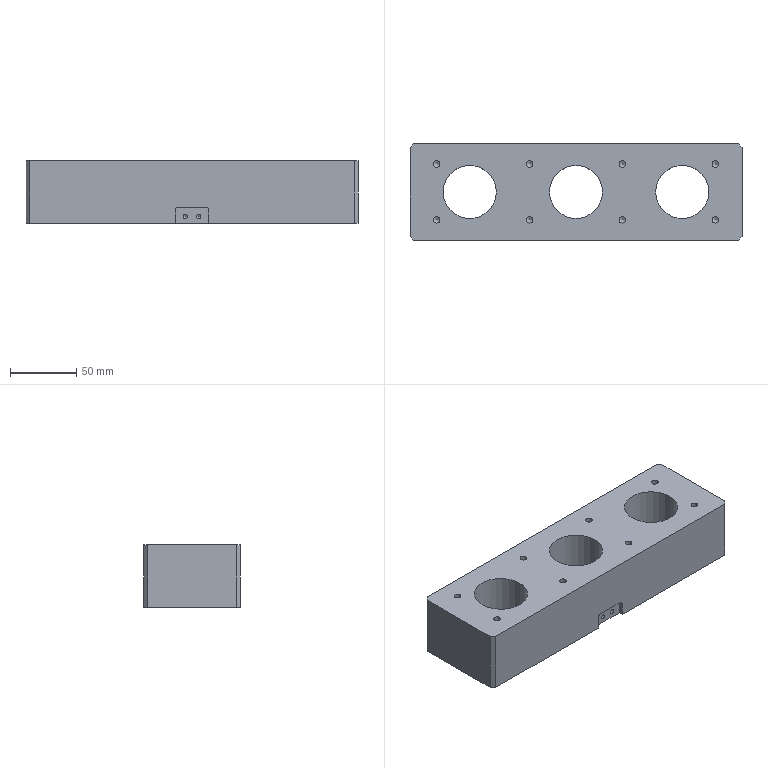Part | NX | 1 solid | 55 faces | box 250 x 73 x 47 mm | volume 670250 mm3 | cylinder 23 | cone 18 | plane 14 | commonest cylinder face diameters 5 x8 6.8 x8 40 x3 3.3 x2 4 x2
STEP:
#1=CARTESIAN_POINT('',(12.5,-36.5,0.));
#2=VERTEX_POINT('',#1);
#3=CARTESIAN_POINT('',(122.,-36.5,0.));
#4=VERTEX_POINT('',#3);
#5=CARTESIAN_POINT('',(125.,-36.5,0.));
#6=DIRECTION('',(1.,0.,0.));
#7=VECTOR('',#6,1000.);
#8=LINE('',#5,#7);
#9=EDGE_CURVE('',#2,#4,#8,.T.);
#10=ORIENTED_EDGE('',*,*,#9,.T.);
#11=CARTESIAN_POINT('',(122.,-36.5,47.));
#12=VERTEX_POINT('',#11);
#13=CARTESIAN_POINT('',(122.,-36.5,47.));
#14=DIRECTION('',(0.,0.,1.));
#15=VECTOR('',#14,1000.);
#16=LINE('',#13,#15);
#17=EDGE_CURVE('',#4,#12,#16,.T.);
#18=ORIENTED_EDGE('',*,*,#17,.T.);
#19=CARTESIAN_POINT('',(-122.,-36.5,47.));
#20=VERTEX_POINT('',#19);
#21=CARTESIAN_POINT('',(125.,-36.5,47.));
#22=DIRECTION('',(1.,0.,0.));
#23=VECTOR('',#22,1000.);
#24=LINE('',#21,#23);
#25=EDGE_CURVE('',#20,#12,#24,.T.);
#26=ORIENTED_EDGE('',*,*,#25,.F.);
#27=CARTESIAN_POINT('',(-122.,-36.5,0.));
#28=VERTEX_POINT('',#27);
#29=CARTESIAN_POINT('',(-122.,-36.5,47.));
#30=DIRECTION('',(0.,0.,-1.));
#31=VECTOR('',#30,1000.);
#32=LINE('',#29,#31);
#33=EDGE_CURVE('',#20,#28,#32,.T.);
#34=ORIENTED_EDGE('',*,*,#33,.T.);
#35=CARTESIAN_POINT('',(-12.5,-36.5,0.));
#36=VERTEX_POINT('',#35);
#37=CARTESIAN_POINT('',(125.,-36.5,0.));
#38=DIRECTION('',(1.,0.,0.));
#39=VECTOR('',#38,1000.);
#40=LINE('',#37,#39);
#41=EDGE_CURVE('',#28,#36,#40,.T.);
#42=ORIENTED_EDGE('',*,*,#41,.T.);
#43=CARTESIAN_POINT('',(-12.5,-36.5,10.));
#44=VERTEX_POINT('',#43);
#45=CARTESIAN_POINT('',(-12.5,-36.5,-12.));
#46=DIRECTION('',(0.,0.,1.));
#47=VECTOR('',#46,1000.);
#48=LINE('',#45,#47);
#49=EDGE_CURVE('',#36,#44,#48,.T.);
#50=ORIENTED_EDGE('',*,*,#49,.T.);
#51=CARTESIAN_POINT('',(-10.5,-36.5,12.));
#52=VERTEX_POINT('',#51);
#53=CARTESIAN_POINT('',(-10.5,-36.5,10.));
#54=DIRECTION('',(0.,1.,0.));
#55=DIRECTION('',(-1.,0.,0.));
#56=AXIS2_PLACEMENT_3D('',#53,#54,#55);
#57=CIRCLE('',#56,2.);
#58=EDGE_CURVE('',#44,#52,#57,.T.);
#59=ORIENTED_EDGE('',*,*,#58,.T.);
#60=CARTESIAN_POINT('',(10.5,-36.5,12.));
#61=VERTEX_POINT('',#60);
#62=CARTESIAN_POINT('',(12.5,-36.5,12.));
#63=DIRECTION('',(1.,0.,0.));
#64=VECTOR('',#63,1000.);
#65=LINE('',#62,#64);
#66=EDGE_CURVE('',#52,#61,#65,.T.);
#67=ORIENTED_EDGE('',*,*,#66,.T.);
#68=CARTESIAN_POINT('',(12.5,-36.5,10.));
#69=VERTEX_POINT('',#68);
#70=CARTESIAN_POINT('',(10.5,-36.5,10.));
#71=DIRECTION('',(0.,1.,0.));
#72=DIRECTION('',(-1.,0.,0.));
#73=AXIS2_PLACEMENT_3D('',#70,#71,#72);
#74=CIRCLE('',#73,2.);
#75=EDGE_CURVE('',#61,#69,#74,.T.);
#76=ORIENTED_EDGE('',*,*,#75,.T.);
#77=CARTESIAN_POINT('',(12.5,-36.5,-12.));
#78=DIRECTION('',(0.,0.,-1.));
#79=VECTOR('',#78,1000.);
#80=LINE('',#77,#79);
#81=EDGE_CURVE('',#69,#2,#80,.T.);
#82=ORIENTED_EDGE('',*,*,#81,.T.);
#83=EDGE_LOOP('',(#10,#18,#26,#34,#42,#50,#59,#67,#76,#82));
#84=FACE_BOUND('',#83,.T.);
#85=CARTESIAN_POINT('',(125.,-36.5,47.));
#86=DIRECTION('',(0.,1.,0.));
#87=DIRECTION('',(-1.,0.,0.));
#88=AXIS2_PLACEMENT_3D('',#85,#86,#87);
#89=PLANE('',#88);
#90=ADVANCED_FACE('',(#84),#89,.F.);
#91=CARTESIAN_POINT('',(102.1,-28.5,0.));
#92=VERTEX_POINT('',#91);
#93=CARTESIAN_POINT('',(105.5,-28.5,0.));
#94=DIRECTION('',(0.,0.,-1.));
#95=DIRECTION('',(-1.,0.,0.));
#96=AXIS2_PLACEMENT_3D('',#93,#94,#95);
#97=CIRCLE('',#96,3.4);
#98=EDGE_CURVE('',#92,#92,#97,.T.);
#99=ORIENTED_EDGE('',*,*,#98,.F.);
#100=EDGE_LOOP('',(#99));
#101=FACE_BOUND('',#100,.T.);
#102=CARTESIAN_POINT('',(57.1,-28.5,0.));
#103=VERTEX_POINT('',#102);
#104=CARTESIAN_POINT('',(60.5,-28.5,0.));
#105=DIRECTION('',(0.,0.,-1.));
#106=DIRECTION('',(-1.,0.,0.));
#107=AXIS2_PLACEMENT_3D('',#104,#105,#106);
#108=CIRCLE('',#107,3.4);
#109=EDGE_CURVE('',#103,#103,#108,.T.);
#110=ORIENTED_EDGE('',*,*,#109,.F.);
#111=EDGE_LOOP('',(#110));
#112=FACE_BOUND('',#111,.T.);
#113=CARTESIAN_POINT('',(-63.9,-28.5,0.));
#114=VERTEX_POINT('',#113);
#115=CARTESIAN_POINT('',(-60.5,-28.5,0.));
#116=DIRECTION('',(0.,0.,-1.));
#117=DIRECTION('',(-1.,0.,0.));
#118=AXIS2_PLACEMENT_3D('',#115,#116,#117);
#119=CIRCLE('',#118,3.4);
#120=EDGE_CURVE('',#114,#114,#119,.T.);
#121=ORIENTED_EDGE('',*,*,#120,.F.);
#122=EDGE_LOOP('',(#121));
#123=FACE_BOUND('',#122,.T.);
#124=CARTESIAN_POINT('',(-108.9,-28.5,0.));
#125=VERTEX_POINT('',#124);
#126=CARTESIAN_POINT('',(-105.5,-28.5,0.));
#127=DIRECTION('',(0.,0.,-1.));
#128=DIRECTION('',(-1.,0.,0.));
#129=AXIS2_PLACEMENT_3D('',#126,#127,#128);
#130=CIRCLE('',#129,3.4);
#131=EDGE_CURVE('',#125,#125,#130,.T.);
#132=ORIENTED_EDGE('',*,*,#131,.F.);
#133=EDGE_LOOP('',(#132));
#134=FACE_BOUND('',#133,.T.);
#135=CARTESIAN_POINT('',(-108.9,28.5,0.));
#136=VERTEX_POINT('',#135);
#137=CARTESIAN_POINT('',(-105.5,28.5,0.));
#138=DIRECTION('',(0.,0.,-1.));
#139=DIRECTION('',(-1.,0.,0.));
#140=AXIS2_PLACEMENT_3D('',#137,#138,#139);
#141=CIRCLE('',#140,3.4);
#142=EDGE_CURVE('',#136,#136,#141,.T.);
#143=ORIENTED_EDGE('',*,*,#142,.F.);
#144=EDGE_LOOP('',(#143));
#145=FACE_BOUND('',#144,.T.);
#146=CARTESIAN_POINT('',(-63.9,28.5,0.));
#147=VERTEX_POINT('',#146);
#148=CARTESIAN_POINT('',(-60.5,28.5,0.));
#149=DIRECTION('',(0.,0.,-1.));
#150=DIRECTION('',(-1.,0.,0.));
#151=AXIS2_PLACEMENT_3D('',#148,#149,#150);
#152=CIRCLE('',#151,3.4);
#153=EDGE_CURVE('',#147,#147,#152,.T.);
#154=ORIENTED_EDGE('',*,*,#153,.F.);
#155=EDGE_LOOP('',(#154));
#156=FACE_BOUND('',#155,.T.);
#157=CARTESIAN_POINT('',(57.1,28.5,0.));
#158=VERTEX_POINT('',#157);
#159=CARTESIAN_POINT('',(60.5,28.5,0.));
#160=DIRECTION('',(0.,0.,-1.));
#161=DIRECTION('',(-1.,0.,0.));
#162=AXIS2_PLACEMENT_3D('',#159,#160,#161);
#163=CIRCLE('',#162,3.4);
#164=EDGE_CURVE('',#158,#158,#163,.T.);
#165=ORIENTED_EDGE('',*,*,#164,.F.);
#166=EDGE_LOOP('',(#165));
#167=FACE_BOUND('',#166,.T.);
#168=CARTESIAN_POINT('',(102.1,28.5,0.));
#169=VERTEX_POINT('',#168);
#170=CARTESIAN_POINT('',(105.5,28.5,0.));
#171=DIRECTION('',(0.,0.,-1.));
#172=DIRECTION('',(-1.,0.,0.));
#173=AXIS2_PLACEMENT_3D('',#170,#171,#172);
#174=CIRCLE('',#173,3.4);
#175=EDGE_CURVE('',#169,#169,#174,.T.);
#176=ORIENTED_EDGE('',*,*,#175,.F.);
#177=EDGE_LOOP('',(#176));
#178=FACE_BOUND('',#177,.T.);
#179=CARTESIAN_POINT('',(-20.,0.,0.));
#180=VERTEX_POINT('',#179);
#181=CARTESIAN_POINT('',(0.,0.,0.));
#182=DIRECTION('',(0.,0.,-1.));
#183=DIRECTION('',(-1.,0.,0.));
#184=AXIS2_PLACEMENT_3D('',#181,#182,#183);
#185=CIRCLE('',#184,20.);
#186=EDGE_CURVE('',#180,#180,#185,.T.);
#187=ORIENTED_EDGE('',*,*,#186,.F.);
#188=EDGE_LOOP('',(#187));
#189=FACE_BOUND('',#188,.T.);
#190=CARTESIAN_POINT('',(-100.,0.,0.));
#191=VERTEX_POINT('',#190);
#192=CARTESIAN_POINT('',(-80.,0.,0.));
#193=DIRECTION('',(0.,0.,-1.));
#194=DIRECTION('',(-1.,0.,0.));
#195=AXIS2_PLACEMENT_3D('',#192,#193,#194);
#196=CIRCLE('',#195,20.);
#197=EDGE_CURVE('',#191,#191,#196,.T.);
#198=ORIENTED_EDGE('',*,*,#197,.F.);
#199=EDGE_LOOP('',(#198));
#200=FACE_BOUND('',#199,.T.);
#201=CARTESIAN_POINT('',(60.,0.,0.));
#202=VERTEX_POINT('',#201);
#203=CARTESIAN_POINT('',(80.,0.,0.));
#204=DIRECTION('',(0.,0.,-1.));
#205=DIRECTION('',(-1.,0.,0.));
#206=AXIS2_PLACEMENT_3D('',#203,#204,#205);
#207=CIRCLE('',#206,20.);
#208=EDGE_CURVE('',#202,#202,#207,.T.);
#209=ORIENTED_EDGE('',*,*,#208,.F.);
#210=EDGE_LOOP('',(#209));
#211=FACE_BOUND('',#210,.T.);
#212=CARTESIAN_POINT('',(122.,36.5,0.));
#213=VERTEX_POINT('',#212);
#214=CARTESIAN_POINT('',(-122.,36.5,0.));
#215=VERTEX_POINT('',#214);
#216=CARTESIAN_POINT('',(125.,36.5,0.));
#217=DIRECTION('',(-1.,0.,0.));
#218=VECTOR('',#217,1000.);
#219=LINE('',#216,#218);
#220=EDGE_CURVE('',#213,#215,#219,.T.);
#221=ORIENTED_EDGE('',*,*,#220,.F.);
#222=CARTESIAN_POINT('',(125.,33.5,0.));
#223=VERTEX_POINT('',#222);
#224=CARTESIAN_POINT('',(79.25,79.25,0.));
#225=DIRECTION('',(-0.7071,0.7071,0.));
#226=VECTOR('',#225,1000.);
#227=LINE('',#224,#226);
#228=EDGE_CURVE('',#213,#223,#227,.F.);
#229=ORIENTED_EDGE('',*,*,#228,.T.);
#230=CARTESIAN_POINT('',(125.,-33.5,0.));
#231=VERTEX_POINT('',#230);
#232=CARTESIAN_POINT('',(125.,36.5,0.));
#233=DIRECTION('',(0.,1.,0.));
#234=VECTOR('',#233,1000.);
#235=LINE('',#232,#234);
#236=EDGE_CURVE('',#231,#223,#235,.T.);
#237=ORIENTED_EDGE('',*,*,#236,.F.);
#238=CARTESIAN_POINT('',(79.25,-79.25,0.));
#239=DIRECTION('',(0.7071,0.7071,0.));
#240=VECTOR('',#239,1000.);
#241=LINE('',#238,#240);
#242=EDGE_CURVE('',#231,#4,#241,.F.);
#243=ORIENTED_EDGE('',*,*,#242,.T.);
#244=ORIENTED_EDGE('',*,*,#9,.F.);
#245=CARTESIAN_POINT('',(12.5,-33.5,0.));
#246=VERTEX_POINT('',#245);
#247=CARTESIAN_POINT('',(12.5,0.,0.));
#248=DIRECTION('',(0.,1.,0.));
#249=VECTOR('',#248,1000.);
#250=LINE('',#247,#249);
#251=EDGE_CURVE('',#2,#246,#250,.T.);
#252=ORIENTED_EDGE('',*,*,#251,.T.);
#253=CARTESIAN_POINT('',(-12.5,-33.5,0.));
#254=VERTEX_POINT('',#253);
#255=CARTESIAN_POINT('',(0.,-33.5,0.));
#256=DIRECTION('',(-1.,0.,0.));
#257=VECTOR('',#256,1000.);
#258=LINE('',#255,#257);
#259=EDGE_CURVE('',#246,#254,#258,.T.);
#260=ORIENTED_EDGE('',*,*,#259,.T.);
#261=CARTESIAN_POINT('',(-12.5,0.,0.));
#262=DIRECTION('',(0.,-1.,0.));
#263=VECTOR('',#262,1000.);
#264=LINE('',#261,#263);
#265=EDGE_CURVE('',#254,#36,#264,.T.);
#266=ORIENTED_EDGE('',*,*,#265,.T.);
#267=ORIENTED_EDGE('',*,*,#41,.F.);
#268=CARTESIAN_POINT('',(-125.,-33.5,0.));
#269=VERTEX_POINT('',#268);
#270=CARTESIAN_POINT('',(-79.25,-79.25,0.));
#271=DIRECTION('',(0.7071,-0.7071,0.));
#272=VECTOR('',#271,1000.);
#273=LINE('',#270,#272);
#274=EDGE_CURVE('',#28,#269,#273,.F.);
#275=ORIENTED_EDGE('',*,*,#274,.T.);
#276=CARTESIAN_POINT('',(-125.,33.5,0.));
#277=VERTEX_POINT('',#276);
#278=CARTESIAN_POINT('',(-125.,36.5,0.));
#279=DIRECTION('',(0.,-1.,0.));
#280=VECTOR('',#279,1000.);
#281=LINE('',#278,#280);
#282=EDGE_CURVE('',#277,#269,#281,.T.);
#283=ORIENTED_EDGE('',*,*,#282,.F.);
#284=CARTESIAN_POINT('',(-79.25,79.25,0.));
#285=DIRECTION('',(-0.7071,-0.7071,0.));
#286=VECTOR('',#285,1000.);
#287=LINE('',#284,#286);
#288=EDGE_CURVE('',#277,#215,#287,.F.);
#289=ORIENTED_EDGE('',*,*,#288,.T.);
#290=EDGE_LOOP('',(#221,#229,#237,#243,#244,#252,#260,#266,#267,#275,#283,#289));
#291=FACE_BOUND('',#290,.T.);
#292=CARTESIAN_POINT('',(0.,0.,0.));
#293=DIRECTION('',(0.,0.,-1.));
#294=DIRECTION('',(-1.,0.,0.));
#295=AXIS2_PLACEMENT_3D('',#292,#293,#294);
#296=PLANE('',#295);
#297=ADVANCED_FACE('',(#101,#112,#123,#134,#145,#156,#167,#178,#189,#200,#211,#291),#296,.T.);
#298=CARTESIAN_POINT('',(-125.,33.5,47.));
#299=VERTEX_POINT('',#298);
#300=CARTESIAN_POINT('',(-125.,-33.5,47.));
#301=VERTEX_POINT('',#300);
#302=CARTESIAN_POINT('',(-125.,36.5,47.));
#303=DIRECTION('',(0.,-1.,0.));
#304=VECTOR('',#303,1000.);
#305=LINE('',#302,#304);
#306=EDGE_CURVE('',#299,#301,#305,.T.);
#307=ORIENTED_EDGE('',*,*,#306,.F.);
#308=CARTESIAN_POINT('',(-125.,33.5,47.));
#309=DIRECTION('',(0.,0.,-1.));
#310=VECTOR('',#309,1000.);
#311=LINE('',#308,#310);
#312=EDGE_CURVE('',#299,#277,#311,.T.);
#313=ORIENTED_EDGE('',*,*,#312,.T.);
#314=ORIENTED_EDGE('',*,*,#282,.T.);
#315=CARTESIAN_POINT('',(-125.,-33.5,47.));
#316=DIRECTION('',(0.,0.,1.));
#317=VECTOR('',#316,1000.);
#318=LINE('',#315,#317);
#319=EDGE_CURVE('',#269,#301,#318,.T.);
#320=ORIENTED_EDGE('',*,*,#319,.T.);
#321=EDGE_LOOP('',(#307,#313,#314,#320));
#322=FACE_BOUND('',#321,.T.);
#323=CARTESIAN_POINT('',(-125.,36.5,47.));
#324=DIRECTION('',(1.,0.,0.));
#325=DIRECTION('',(0.,1.,0.));
#326=AXIS2_PLACEMENT_3D('',#323,#324,#325);
#327=PLANE('',#326);
#328=ADVANCED_FACE('',(#322),#327,.F.);
#329=ORIENTED_EDGE('',*,*,#236,.T.);
#330=CARTESIAN_POINT('',(125.,33.5,47.));
#331=VERTEX_POINT('',#330);
#332=CARTESIAN_POINT('',(125.,33.5,47.));
#333=DIRECTION('',(0.,0.,1.));
#334=VECTOR('',#333,1000.);
#335=LINE('',#332,#334);
#336=EDGE_CURVE('',#223,#331,#335,.T.);
#337=ORIENTED_EDGE('',*,*,#336,.T.);
#338=CARTESIAN_POINT('',(125.,-33.5,47.));
#339=VERTEX_POINT('',#338);
#340=CARTESIAN_POINT('',(125.,36.5,47.));
#341=DIRECTION('',(0.,1.,0.));
#342=VECTOR('',#341,1000.);
#343=LINE('',#340,#342);
#344=EDGE_CURVE('',#339,#331,#343,.T.);
#345=ORIENTED_EDGE('',*,*,#344,.F.);
#346=CARTESIAN_POINT('',(125.,-33.5,47.));
#347=DIRECTION('',(0.,0.,-1.));
#348=VECTOR('',#347,1000.);
#349=LINE('',#346,#348);
#350=EDGE_CURVE('',#339,#231,#349,.T.);
#351=ORIENTED_EDGE('',*,*,#350,.T.);
#352=EDGE_LOOP('',(#329,#337,#345,#351));
#353=FACE_BOUND('',#352,.T.);
#354=CARTESIAN_POINT('',(125.,36.5,47.));
#355=DIRECTION('',(-1.,0.,0.));
#356=DIRECTION('',(0.,0.,1.));
#357=AXIS2_PLACEMENT_3D('',#354,#355,#356);
#358=PLANE('',#357);
#359=ADVANCED_FACE('',(#353),#358,.F.);
#360=CARTESIAN_POINT('',(122.,36.5,47.));
#361=VERTEX_POINT('',#360);
#362=CARTESIAN_POINT('',(-122.,36.5,47.));
#363=VERTEX_POINT('',#362);
#364=CARTESIAN_POINT('',(125.,36.5,47.));
#365=DIRECTION('',(-1.,0.,0.));
#366=VECTOR('',#365,1000.);
#367=LINE('',#364,#366);
#368=EDGE_CURVE('',#361,#363,#367,.T.);
#369=ORIENTED_EDGE('',*,*,#368,.F.);
#370=CARTESIAN_POINT('',(122.,36.5,47.));
#371=DIRECTION('',(0.,0.,-1.));
#372=VECTOR('',#371,1000.);
#373=LINE('',#370,#372);
#374=EDGE_CURVE('',#361,#213,#373,.T.);
#375=ORIENTED_EDGE('',*,*,#374,.T.);
#376=ORIENTED_EDGE('',*,*,#220,.T.);
#377=CARTESIAN_POINT('',(-122.,36.5,47.));
#378=DIRECTION('',(0.,0.,1.));
#379=VECTOR('',#378,1000.);
#380=LINE('',#377,#379);
#381=EDGE_CURVE('',#215,#363,#380,.T.);
#382=ORIENTED_EDGE('',*,*,#381,.T.);
#383=EDGE_LOOP('',(#369,#375,#376,#382));
#384=FACE_BOUND('',#383,.T.);
#385=CARTESIAN_POINT('',(125.,36.5,47.));
#386=DIRECTION('',(0.,-1.,0.));
#387=DIRECTION('',(1.,0.,0.));
#388=AXIS2_PLACEMENT_3D('',#385,#386,#387);
#389=PLANE('',#388);
#390=ADVANCED_FACE('',(#384),#389,.F.);
#391=CARTESIAN_POINT('',(60.,0.,47.));
#392=VERTEX_POINT('',#391);
#393=CARTESIAN_POINT('',(80.,0.,47.));
#394=DIRECTION('',(0.,0.,-1.));
#395=DIRECTION('',(-1.,0.,0.));
#396=AXIS2_PLACEMENT_3D('',#393,#394,#395);
#397=CIRCLE('',#396,20.);
#398=EDGE_CURVE('',#392,#392,#397,.T.);
#399=ORIENTED_EDGE('',*,*,#398,.T.);
#400=EDGE_LOOP('',(#399));
#401=FACE_BOUND('',#400,.T.);
#402=CARTESIAN_POINT('',(-100.,0.,47.));
#403=VERTEX_POINT('',#402);
#404=CARTESIAN_POINT('',(-80.,0.,47.));
#405=DIRECTION('',(0.,0.,-1.));
#406=DIRECTION('',(-1.,0.,0.));
#407=AXIS2_PLACEMENT_3D('',#404,#405,#406);
#408=CIRCLE('',#407,20.);
#409=EDGE_CURVE('',#403,#403,#408,.T.);
#410=ORIENTED_EDGE('',*,*,#409,.T.);
#411=EDGE_LOOP('',(#410));
#412=FACE_BOUND('',#411,.T.);
#413=CARTESIAN_POINT('',(-20.,0.,47.));
#414=VERTEX_POINT('',#413);
#415=CARTESIAN_POINT('',(0.,0.,47.));
#416=DIRECTION('',(0.,0.,-1.));
#417=DIRECTION('',(-1.,0.,0.));
#418=AXIS2_PLACEMENT_3D('',#415,#416,#417);
#419=CIRCLE('',#418,20.);
#420=EDGE_CURVE('',#414,#414,#419,.T.);
#421=ORIENTED_EDGE('',*,*,#420,.T.);
#422=EDGE_LOOP('',(#421));
#423=FACE_BOUND('',#422,.T.);
#424=CARTESIAN_POINT('',(-102.5,21.,47.));
#425=VERTEX_POINT('',#424);
#426=CARTESIAN_POINT('',(-105.,21.,47.));
#427=DIRECTION('',(0.,0.,1.));
#428=DIRECTION('',(1.,0.,0.));
#429=AXIS2_PLACEMENT_3D('',#426,#427,#428);
#430=CIRCLE('',#429,2.5);
#431=EDGE_CURVE('',#425,#425,#430,.T.);
#432=ORIENTED_EDGE('',*,*,#431,.F.);
#433=EDGE_LOOP('',(#432));
#434=FACE_BOUND('',#433,.T.);
#435=CARTESIAN_POINT('',(-32.5,21.,47.));
#436=VERTEX_POINT('',#435);
#437=CARTESIAN_POINT('',(-35.,21.,47.));
#438=DIRECTION('',(0.,0.,1.));
#439=DIRECTION('',(1.,0.,0.));
#440=AXIS2_PLACEMENT_3D('',#437,#438,#439);
#441=CIRCLE('',#440,2.5);
#442=EDGE_CURVE('',#436,#436,#441,.T.);
#443=ORIENTED_EDGE('',*,*,#442,.F.);
#444=EDGE_LOOP('',(#443));
#445=FACE_BOUND('',#444,.T.);
#446=CARTESIAN_POINT('',(-32.5,-21.,47.));
#447=VERTEX_POINT('',#446);
#448=CARTESIAN_POINT('',(-35.,-21.,47.));
#449=DIRECTION('',(0.,0.,1.));
#450=DIRECTION('',(1.,0.,0.));
#451=AXIS2_PLACEMENT_3D('',#448,#449,#450);
#452=CIRCLE('',#451,2.5);
#453=EDGE_CURVE('',#447,#447,#452,.T.);
#454=ORIENTED_EDGE('',*,*,#453,.F.);
#455=EDGE_LOOP('',(#454));
#456=FACE_BOUND('',#455,.T.);
#457=CARTESIAN_POINT('',(-102.5,-21.,47.));
#458=VERTEX_POINT('',#457);
#459=CARTESIAN_POINT('',(-105.,-21.,47.));
#460=DIRECTION('',(0.,0.,1.));
#461=DIRECTION('',(1.,0.,0.));
#462=AXIS2_PLACEMENT_3D('',#459,#460,#461);
#463=CIRCLE('',#462,2.5);
#464=EDGE_CURVE('',#458,#458,#463,.T.);
#465=ORIENTED_EDGE('',*,*,#464,.F.);
#466=EDGE_LOOP('',(#465));
#467=FACE_BOUND('',#466,.T.);
#468=CARTESIAN_POINT('',(107.5,-21.,47.));
#469=VERTEX_POINT('',#468);
#470=CARTESIAN_POINT('',(105.,-21.,47.));
#471=DIRECTION('',(0.,0.,1.));
#472=DIRECTION('',(1.,0.,0.));
#473=AXIS2_PLACEMENT_3D('',#470,#471,#472);
#474=CIRCLE('',#473,2.5);
#475=EDGE_CURVE('',#469,#469,#474,.T.);
#476=ORIENTED_EDGE('',*,*,#475,.F.);
#477=EDGE_LOOP('',(#476));
#478=FACE_BOUND('',#477,.T.);
#479=CARTESIAN_POINT('',(37.5,-21.,47.));
#480=VERTEX_POINT('',#479);
#481=CARTESIAN_POINT('',(35.,-21.,47.));
#482=DIRECTION('',(0.,0.,1.));
#483=DIRECTION('',(1.,0.,0.));
#484=AXIS2_PLACEMENT_3D('',#481,#482,#483);
#485=CIRCLE('',#484,2.5);
#486=EDGE_CURVE('',#480,#480,#485,.T.);
#487=ORIENTED_EDGE('',*,*,#486,.F.);
#488=EDGE_LOOP('',(#487));
#489=FACE_BOUND('',#488,.T.);
#490=CARTESIAN_POINT('',(37.5,21.,47.));
#491=VERTEX_POINT('',#490);
#492=CARTESIAN_POINT('',(35.,21.,47.));
#493=DIRECTION('',(0.,0.,1.));
#494=DIRECTION('',(1.,0.,0.));
#495=AXIS2_PLACEMENT_3D('',#492,#493,#494);
#496=CIRCLE('',#495,2.5);
#497=EDGE_CURVE('',#491,#491,#496,.T.);
#498=ORIENTED_EDGE('',*,*,#497,.F.);
#499=EDGE_LOOP('',(#498));
#500=FACE_BOUND('',#499,.T.);
#501=CARTESIAN_POINT('',(107.5,21.,47.));
#502=VERTEX_POINT('',#501);
#503=CARTESIAN_POINT('',(105.,21.,47.));
#504=DIRECTION('',(0.,0.,1.));
#505=DIRECTION('',(1.,0.,0.));
#506=AXIS2_PLACEMENT_3D('',#503,#504,#505);
#507=CIRCLE('',#506,2.5);
#508=EDGE_CURVE('',#502,#502,#507,.T.);
#509=ORIENTED_EDGE('',*,*,#508,.F.);
#510=EDGE_LOOP('',(#509));
#511=FACE_BOUND('',#510,.T.);
#512=ORIENTED_EDGE('',*,*,#344,.T.);
#513=CARTESIAN_POINT('',(122.,36.5,47.));
#514=DIRECTION('',(0.7071,-0.7071,0.));
#515=VECTOR('',#514,1000.);
#516=LINE('',#513,#515);
#517=EDGE_CURVE('',#331,#361,#516,.F.);
#518=ORIENTED_EDGE('',*,*,#517,.T.);
#519=ORIENTED_EDGE('',*,*,#368,.T.);
#520=CARTESIAN_POINT('',(-125.,33.5,47.));
#521=DIRECTION('',(0.7071,0.7071,0.));
#522=VECTOR('',#521,1000.);
#523=LINE('',#520,#522);
#524=EDGE_CURVE('',#363,#299,#523,.F.);
#525=ORIENTED_EDGE('',*,*,#524,.T.);
#526=ORIENTED_EDGE('',*,*,#306,.T.);
#527=CARTESIAN_POINT('',(-122.,-36.5,47.));
#528=DIRECTION('',(-0.7071,0.7071,0.));
#529=VECTOR('',#528,1000.);
#530=LINE('',#527,#529);
#531=EDGE_CURVE('',#301,#20,#530,.F.);
#532=ORIENTED_EDGE('',*,*,#531,.T.);
#533=ORIENTED_EDGE('',*,*,#25,.T.);
#534=CARTESIAN_POINT('',(125.,-33.5,47.));
#535=DIRECTION('',(-0.7071,-0.7071,0.));
#536=VECTOR('',#535,1000.);
#537=LINE('',#534,#536);
#538=EDGE_CURVE('',#12,#339,#537,.F.);
#539=ORIENTED_EDGE('',*,*,#538,.T.);
#540=EDGE_LOOP('',(#512,#518,#519,#525,#526,#532,#533,#539));
#541=FACE_BOUND('',#540,.T.);
#542=CARTESIAN_POINT('',(0.,0.,47.));
#543=DIRECTION('',(0.,0.,-1.));
#544=DIRECTION('',(-1.,0.,0.));
#545=AXIS2_PLACEMENT_3D('',#542,#543,#544);
#546=PLANE('',#545);
#547=ADVANCED_FACE('',(#401,#412,#423,#434,#445,#456,#467,#478,#489,#500,#511,#541),#546,.F.);
#548=CARTESIAN_POINT('',(105.5,-28.5,21.793));
#549=VERTEX_POINT('',#548);
#550=VERTEX_LOOP('',#549);
#551=FACE_BOUND('',#550,.T.);
#552=CARTESIAN_POINT('',(102.1,-28.5,19.75));
#553=VERTEX_POINT('',#552);
#554=CARTESIAN_POINT('',(105.5,-28.5,19.75));
#555=DIRECTION('',(0.,0.,-1.));
#556=DIRECTION('',(-1.,0.,0.));
#557=AXIS2_PLACEMENT_3D('',#554,#555,#556);
#558=CIRCLE('',#557,3.4);
#559=EDGE_CURVE('',#553,#553,#558,.T.);
#560=ORIENTED_EDGE('',*,*,#559,.T.);
#561=EDGE_LOOP('',(#560));
#562=FACE_BOUND('',#561,.T.);
#563=CARTESIAN_POINT('',(105.5,-28.5,19.75));
#564=DIRECTION('',(0.,0.,-1.));
#565=DIRECTION('',(-1.,0.,0.));
#566=AXIS2_PLACEMENT_3D('',#563,#564,#565);
#567=CONICAL_SURFACE('',#566,3.4,1.03);
#568=ADVANCED_FACE('',(#551,#562),#567,.F.);
#569=ORIENTED_EDGE('',*,*,#559,.F.);
#570=EDGE_LOOP('',(#569));
#571=FACE_BOUND('',#570,.T.);
#572=ORIENTED_EDGE('',*,*,#98,.T.);
#573=EDGE_LOOP('',(#572));
#574=FACE_BOUND('',#573,.T.);
#575=CARTESIAN_POINT('',(105.5,-28.5,0.));
#576=DIRECTION('',(0.,0.,-1.));
#577=DIRECTION('',(-1.,0.,0.));
#578=AXIS2_PLACEMENT_3D('',#575,#576,#577);
#579=CYLINDRICAL_SURFACE('',#578,3.4);
#580=ADVANCED_FACE('',(#571,#574),#579,.F.);
#581=CARTESIAN_POINT('',(60.5,-28.5,21.793));
#582=VERTEX_POINT('',#581);
#583=VERTEX_LOOP('',#582);
#584=FACE_BOUND('',#583,.T.);
#585=CARTESIAN_POINT('',(57.1,-28.5,19.75));
#586=VERTEX_POINT('',#585);
#587=CARTESIAN_POINT('',(60.5,-28.5,19.75));
#588=DIRECTION('',(0.,0.,-1.));
#589=DIRECTION('',(-1.,0.,0.));
#590=AXIS2_PLACEMENT_3D('',#587,#588,#589);
#591=CIRCLE('',#590,3.4);
#592=EDGE_CURVE('',#586,#586,#591,.T.);
#593=ORIENTED_EDGE('',*,*,#592,.T.);
#594=EDGE_LOOP('',(#593));
#595=FACE_BOUND('',#594,.T.);
#596=CARTESIAN_POINT('',(60.5,-28.5,19.75));
#597=DIRECTION('',(0.,0.,-1.));
#598=DIRECTION('',(-1.,0.,0.));
#599=AXIS2_PLACEMENT_3D('',#596,#597,#598);
#600=CONICAL_SURFACE('',#599,3.4,1.03);
#601=ADVANCED_FACE('',(#584,#595),#600,.F.);
#602=ORIENTED_EDGE('',*,*,#592,.F.);
#603=EDGE_LOOP('',(#602));
#604=FACE_BOUND('',#603,.T.);
#605=ORIENTED_EDGE('',*,*,#109,.T.);
#606=EDGE_LOOP('',(#605));
#607=FACE_BOUND('',#606,.T.);
#608=CARTESIAN_POINT('',(60.5,-28.5,0.));
#609=DIRECTION('',(0.,0.,-1.));
#610=DIRECTION('',(-1.,0.,0.));
#611=AXIS2_PLACEMENT_3D('',#608,#609,#610);
#612=CYLINDRICAL_SURFACE('',#611,3.4);
#613=ADVANCED_FACE('',(#604,#607),#612,.F.);
#614=CARTESIAN_POINT('',(-60.5,-28.5,21.793));
#615=VERTEX_POINT('',#614);
#616=VERTEX_LOOP('',#615);
#617=FACE_BOUND('',#616,.T.);
#618=CARTESIAN_POINT('',(-63.9,-28.5,19.75));
#619=VERTEX_POINT('',#618);
#620=CARTESIAN_POINT('',(-60.5,-28.5,19.75));
#621=DIRECTION('',(0.,0.,-1.));
#622=DIRECTION('',(-1.,0.,0.));
#623=AXIS2_PLACEMENT_3D('',#620,#621,#622);
#624=CIRCLE('',#623,3.4);
#625=EDGE_CURVE('',#619,#619,#624,.T.);
#626=ORIENTED_EDGE('',*,*,#625,.T.);
#627=EDGE_LOOP('',(#626));
#628=FACE_BOUND('',#627,.T.);
#629=CARTESIAN_POINT('',(-60.5,-28.5,19.75));
#630=DIRECTION('',(0.,0.,-1.));
#631=DIRECTION('',(-1.,0.,0.));
#632=AXIS2_PLACEMENT_3D('',#629,#630,#631);
#633=CONICAL_SURFACE('',#632,3.4,1.03);
#634=ADVANCED_FACE('',(#617,#628),#633,.F.);
#635=ORIENTED_EDGE('',*,*,#625,.F.);
#636=EDGE_LOOP('',(#635));
#637=FACE_BOUND('',#636,.T.);
#638=ORIENTED_EDGE('',*,*,#120,.T.);
#639=EDGE_LOOP('',(#638));
#640=FACE_BOUND('',#639,.T.);
#641=CARTESIAN_POINT('',(-60.5,-28.5,0.));
#642=DIRECTION('',(0.,0.,-1.));
#643=DIRECTION('',(-1.,0.,0.));
#644=AXIS2_PLACEMENT_3D('',#641,#642,#643);
#645=CYLINDRICAL_SURFACE('',#644,3.4);
#646=ADVANCED_FACE('',(#637,#640),#645,.F.);
#647=CARTESIAN_POINT('',(-105.5,-28.5,21.793));
#648=VERTEX_POINT('',#647);
#649=VERTEX_LOOP('',#648);
#650=FACE_BOUND('',#649,.T.);
#651=CARTESIAN_POINT('',(-108.9,-28.5,19.75));
#652=VERTEX_POINT('',#651);
#653=CARTESIAN_POINT('',(-105.5,-28.5,19.75));
#654=DIRECTION('',(0.,0.,-1.));
#655=DIRECTION('',(-1.,0.,0.));
#656=AXIS2_PLACEMENT_3D('',#653,#654,#655);
#657=CIRCLE('',#656,3.4);
#658=EDGE_CURVE('',#652,#652,#657,.T.);
#659=ORIENTED_EDGE('',*,*,#658,.T.);
#660=EDGE_LOOP('',(#659));
#661=FACE_BOUND('',#660,.T.);
#662=CARTESIAN_POINT('',(-105.5,-28.5,19.75));
#663=DIRECTION('',(0.,0.,-1.));
#664=DIRECTION('',(-1.,0.,0.));
#665=AXIS2_PLACEMENT_3D('',#662,#663,#664);
#666=CONICAL_SURFACE('',#665,3.4,1.03);
#667=ADVANCED_FACE('',(#650,#661),#666,.F.);
#668=ORIENTED_EDGE('',*,*,#658,.F.);
#669=EDGE_LOOP('',(#668));
#670=FACE_BOUND('',#669,.T.);
#671=ORIENTED_EDGE('',*,*,#131,.T.);
#672=EDGE_LOOP('',(#671));
#673=FACE_BOUND('',#672,.T.);
#674=CARTESIAN_POINT('',(-105.5,-28.5,0.));
#675=DIRECTION('',(0.,0.,-1.));
#676=DIRECTION('',(-1.,0.,0.));
#677=AXIS2_PLACEMENT_3D('',#674,#675,#676);
#678=CYLINDRICAL_SURFACE('',#677,3.4);
#679=ADVANCED_FACE('',(#670,#673),#678,.F.);
#680=CARTESIAN_POINT('',(-105.5,28.5,21.793));
#681=VERTEX_POINT('',#680);
#682=VERTEX_LOOP('',#681);
#683=FACE_BOUND('',#682,.T.);
#684=CARTESIAN_POINT('',(-108.9,28.5,19.75));
#685=VERTEX_POINT('',#684);
#686=CARTESIAN_POINT('',(-105.5,28.5,19.75));
#687=DIRECTION('',(0.,0.,-1.));
#688=DIRECTION('',(-1.,0.,0.));
#689=AXIS2_PLACEMENT_3D('',#686,#687,#688);
#690=CIRCLE('',#689,3.4);
#691=EDGE_CURVE('',#685,#685,#690,.T.);
#692=ORIENTED_EDGE('',*,*,#691,.T.);
#693=EDGE_LOOP('',(#692));
#694=FACE_BOUND('',#693,.T.);
#695=CARTESIAN_POINT('',(-105.5,28.5,19.75));
#696=DIRECTION('',(0.,0.,-1.));
#697=DIRECTION('',(-1.,0.,0.));
#698=AXIS2_PLACEMENT_3D('',#695,#696,#697);
#699=CONICAL_SURFACE('',#698,3.4,1.03);
#700=ADVANCED_FACE('',(#683,#694),#699,.F.);
#701=ORIENTED_EDGE('',*,*,#691,.F.);
#702=EDGE_LOOP('',(#701));
#703=FACE_BOUND('',#702,.T.);
#704=ORIENTED_EDGE('',*,*,#142,.T.);
#705=EDGE_LOOP('',(#704));
#706=FACE_BOUND('',#705,.T.);
#707=CARTESIAN_POINT('',(-105.5,28.5,0.));
#708=DIRECTION('',(0.,0.,-1.));
#709=DIRECTION('',(-1.,0.,0.));
#710=AXIS2_PLACEMENT_3D('',#707,#708,#709);
#711=CYLINDRICAL_SURFACE('',#710,3.4);
#712=ADVANCED_FACE('',(#703,#706),#711,.F.);
#713=CARTESIAN_POINT('',(-60.5,28.5,21.793));
#714=VERTEX_POINT('',#713);
#715=VERTEX_LOOP('',#714);
#716=FACE_BOUND('',#715,.T.);
#717=CARTESIAN_POINT('',(-63.9,28.5,19.75));
#718=VERTEX_POINT('',#717);
#719=CARTESIAN_POINT('',(-60.5,28.5,19.75));
#720=DIRECTION('',(0.,0.,-1.));
#721=DIRECTION('',(-1.,0.,0.));
#722=AXIS2_PLACEMENT_3D('',#719,#720,#721);
#723=CIRCLE('',#722,3.4);
#724=EDGE_CURVE('',#718,#718,#723,.T.);
#725=ORIENTED_EDGE('',*,*,#724,.T.);
#726=EDGE_LOOP('',(#725));
#727=FACE_BOUND('',#726,.T.);
#728=CARTESIAN_POINT('',(-60.5,28.5,19.75));
#729=DIRECTION('',(0.,0.,-1.));
#730=DIRECTION('',(-1.,0.,0.));
#731=AXIS2_PLACEMENT_3D('',#728,#729,#730);
#732=CONICAL_SURFACE('',#731,3.4,1.03);
#733=ADVANCED_FACE('',(#716,#727),#732,.F.);
#734=ORIENTED_EDGE('',*,*,#724,.F.);
#735=EDGE_LOOP('',(#734));
#736=FACE_BOUND('',#735,.T.);
#737=ORIENTED_EDGE('',*,*,#153,.T.);
#738=EDGE_LOOP('',(#737));
#739=FACE_BOUND('',#738,.T.);
#740=CARTESIAN_POINT('',(-60.5,28.5,0.));
#741=DIRECTION('',(0.,0.,-1.));
#742=DIRECTION('',(-1.,0.,0.));
#743=AXIS2_PLACEMENT_3D('',#740,#741,#742);
#744=CYLINDRICAL_SURFACE('',#743,3.4);
#745=ADVANCED_FACE('',(#736,#739),#744,.F.);
#746=CARTESIAN_POINT('',(60.5,28.5,21.793));
#747=VERTEX_POINT('',#746);
#748=VERTEX_LOOP('',#747);
#749=FACE_BOUND('',#748,.T.);
#750=CARTESIAN_POINT('',(57.1,28.5,19.75));
#751=VERTEX_POINT('',#750);
#752=CARTESIAN_POINT('',(60.5,28.5,19.75));
#753=DIRECTION('',(0.,0.,-1.));
#754=DIRECTION('',(-1.,0.,0.));
#755=AXIS2_PLACEMENT_3D('',#752,#753,#754);
#756=CIRCLE('',#755,3.4);
#757=EDGE_CURVE('',#751,#751,#756,.T.);
#758=ORIENTED_EDGE('',*,*,#757,.T.);
#759=EDGE_LOOP('',(#758));
#760=FACE_BOUND('',#759,.T.);
#761=CARTESIAN_POINT('',(60.5,28.5,19.75));
#762=DIRECTION('',(0.,0.,-1.));
#763=DIRECTION('',(-1.,0.,0.));
#764=AXIS2_PLACEMENT_3D('',#761,#762,#763);
#765=CONICAL_SURFACE('',#764,3.4,1.03);
#766=ADVANCED_FACE('',(#749,#760),#765,.F.);
#767=ORIENTED_EDGE('',*,*,#757,.F.);
#768=EDGE_LOOP('',(#767));
#769=FACE_BOUND('',#768,.T.);
#770=ORIENTED_EDGE('',*,*,#164,.T.);
#771=EDGE_LOOP('',(#770));
#772=FACE_BOUND('',#771,.T.);
#773=CARTESIAN_POINT('',(60.5,28.5,0.));
#774=DIRECTION('',(0.,0.,-1.));
#775=DIRECTION('',(-1.,0.,0.));
#776=AXIS2_PLACEMENT_3D('',#773,#774,#775);
#777=CYLINDRICAL_SURFACE('',#776,3.4);
#778=ADVANCED_FACE('',(#769,#772),#777,.F.);
#779=CARTESIAN_POINT('',(105.5,28.5,21.793));
#780=VERTEX_POINT('',#779);
#781=VERTEX_LOOP('',#780);
#782=FACE_BOUND('',#781,.T.);
#783=CARTESIAN_POINT('',(102.1,28.5,19.75));
#784=VERTEX_POINT('',#783);
#785=CARTESIAN_POINT('',(105.5,28.5,19.75));
#786=DIRECTION('',(0.,0.,-1.));
#787=DIRECTION('',(-1.,0.,0.));
#788=AXIS2_PLACEMENT_3D('',#785,#786,#787);
#789=CIRCLE('',#788,3.4);
#790=EDGE_CURVE('',#784,#784,#789,.T.);
#791=ORIENTED_EDGE('',*,*,#790,.T.);
#792=EDGE_LOOP('',(#791));
#793=FACE_BOUND('',#792,.T.);
#794=CARTESIAN_POINT('',(105.5,28.5,19.75));
#795=DIRECTION('',(0.,0.,-1.));
#796=DIRECTION('',(-1.,0.,0.));
#797=AXIS2_PLACEMENT_3D('',#794,#795,#796);
#798=CONICAL_SURFACE('',#797,3.4,1.03);
#799=ADVANCED_FACE('',(#782,#793),#798,.F.);
#800=ORIENTED_EDGE('',*,*,#790,.F.);
#801=EDGE_LOOP('',(#800));
#802=FACE_BOUND('',#801,.T.);
#803=ORIENTED_EDGE('',*,*,#175,.T.);
#804=EDGE_LOOP('',(#803));
#805=FACE_BOUND('',#804,.T.);
#806=CARTESIAN_POINT('',(105.5,28.5,0.));
#807=DIRECTION('',(0.,0.,-1.));
#808=DIRECTION('',(-1.,0.,0.));
#809=AXIS2_PLACEMENT_3D('',#806,#807,#808);
#810=CYLINDRICAL_SURFACE('',#809,3.4);
#811=ADVANCED_FACE('',(#802,#805),#810,.F.);
#812=CARTESIAN_POINT('',(105.,21.,30.498));
#813=VERTEX_POINT('',#812);
#814=VERTEX_LOOP('',#813);
#815=FACE_BOUND('',#814,.T.);
#816=CARTESIAN_POINT('',(107.5,21.,32.));
#817=VERTEX_POINT('',#816);
#818=CARTESIAN_POINT('',(105.,21.,32.));
#819=DIRECTION('',(0.,0.,1.));
#820=DIRECTION('',(1.,0.,0.));
#821=AXIS2_PLACEMENT_3D('',#818,#819,#820);
#822=CIRCLE('',#821,2.5);
#823=EDGE_CURVE('',#817,#817,#822,.T.);
#824=ORIENTED_EDGE('',*,*,#823,.T.);
#825=EDGE_LOOP('',(#824));
#826=FACE_BOUND('',#825,.T.);
#827=CARTESIAN_POINT('',(105.,21.,32.));
#828=DIRECTION('',(0.,0.,1.));
#829=DIRECTION('',(1.,0.,0.));
#830=AXIS2_PLACEMENT_3D('',#827,#828,#829);
#831=CONICAL_SURFACE('',#830,2.5,1.03);
#832=ADVANCED_FACE('',(#815,#826),#831,.F.);
#833=ORIENTED_EDGE('',*,*,#823,.F.);
#834=EDGE_LOOP('',(#833));
#835=FACE_BOUND('',#834,.T.);
#836=ORIENTED_EDGE('',*,*,#508,.T.);
#837=EDGE_LOOP('',(#836));
#838=FACE_BOUND('',#837,.T.);
#839=CARTESIAN_POINT('',(105.,21.,47.));
#840=DIRECTION('',(0.,0.,1.));
#841=DIRECTION('',(1.,0.,0.));
#842=AXIS2_PLACEMENT_3D('',#839,#840,#841);
#843=CYLINDRICAL_SURFACE('',#842,2.5);
#844=ADVANCED_FACE('',(#835,#838),#843,.F.);
#845=CARTESIAN_POINT('',(35.,21.,30.498));
#846=VERTEX_POINT('',#845);
#847=VERTEX_LOOP('',#846);
#848=FACE_BOUND('',#847,.T.);
#849=CARTESIAN_POINT('',(37.5,21.,32.));
#850=VERTEX_POINT('',#849);
#851=CARTESIAN_POINT('',(35.,21.,32.));
#852=DIRECTION('',(0.,0.,1.));
#853=DIRECTION('',(1.,0.,0.));
#854=AXIS2_PLACEMENT_3D('',#851,#852,#853);
#855=CIRCLE('',#854,2.5);
#856=EDGE_CURVE('',#850,#850,#855,.T.);
#857=ORIENTED_EDGE('',*,*,#856,.T.);
#858=EDGE_LOOP('',(#857));
#859=FACE_BOUND('',#858,.T.);
#860=CARTESIAN_POINT('',(35.,21.,32.));
#861=DIRECTION('',(0.,0.,1.));
#862=DIRECTION('',(1.,0.,0.));
#863=AXIS2_PLACEMENT_3D('',#860,#861,#862);
#864=CONICAL_SURFACE('',#863,2.5,1.03);
#865=ADVANCED_FACE('',(#848,#859),#864,.F.);
#866=ORIENTED_EDGE('',*,*,#856,.F.);
#867=EDGE_LOOP('',(#866));
#868=FACE_BOUND('',#867,.T.);
#869=ORIENTED_EDGE('',*,*,#497,.T.);
#870=EDGE_LOOP('',(#869));
#871=FACE_BOUND('',#870,.T.);
#872=CARTESIAN_POINT('',(35.,21.,47.));
#873=DIRECTION('',(0.,0.,1.));
#874=DIRECTION('',(1.,0.,0.));
#875=AXIS2_PLACEMENT_3D('',#872,#873,#874);
#876=CYLINDRICAL_SURFACE('',#875,2.5);
#877=ADVANCED_FACE('',(#868,#871),#876,.F.);
#878=CARTESIAN_POINT('',(35.,-21.,30.498));
#879=VERTEX_POINT('',#878);
#880=VERTEX_LOOP('',#879);
#881=FACE_BOUND('',#880,.T.);
#882=CARTESIAN_POINT('',(37.5,-21.,32.));
#883=VERTEX_POINT('',#882);
#884=CARTESIAN_POINT('',(35.,-21.,32.));
#885=DIRECTION('',(0.,0.,1.));
#886=DIRECTION('',(1.,0.,0.));
#887=AXIS2_PLACEMENT_3D('',#884,#885,#886);
#888=CIRCLE('',#887,2.5);
#889=EDGE_CURVE('',#883,#883,#888,.T.);
#890=ORIENTED_EDGE('',*,*,#889,.T.);
#891=EDGE_LOOP('',(#890));
#892=FACE_BOUND('',#891,.T.);
#893=CARTESIAN_POINT('',(35.,-21.,32.));
#894=DIRECTION('',(0.,0.,1.));
#895=DIRECTION('',(1.,0.,0.));
#896=AXIS2_PLACEMENT_3D('',#893,#894,#895);
#897=CONICAL_SURFACE('',#896,2.5,1.03);
#898=ADVANCED_FACE('',(#881,#892),#897,.F.);
#899=ORIENTED_EDGE('',*,*,#889,.F.);
#900=EDGE_LOOP('',(#899));
#901=FACE_BOUND('',#900,.T.);
#902=ORIENTED_EDGE('',*,*,#486,.T.);
#903=EDGE_LOOP('',(#902));
#904=FACE_BOUND('',#903,.T.);
#905=CARTESIAN_POINT('',(35.,-21.,47.));
#906=DIRECTION('',(0.,0.,1.));
#907=DIRECTION('',(1.,0.,0.));
#908=AXIS2_PLACEMENT_3D('',#905,#906,#907);
#909=CYLINDRICAL_SURFACE('',#908,2.5);
#910=ADVANCED_FACE('',(#901,#904),#909,.F.);
#911=CARTESIAN_POINT('',(105.,-21.,30.498));
#912=VERTEX_POINT('',#911);
#913=VERTEX_LOOP('',#912);
#914=FACE_BOUND('',#913,.T.);
#915=CARTESIAN_POINT('',(107.5,-21.,32.));
#916=VERTEX_POINT('',#915);
#917=CARTESIAN_POINT('',(105.,-21.,32.));
#918=DIRECTION('',(0.,0.,1.));
#919=DIRECTION('',(1.,0.,0.));
#920=AXIS2_PLACEMENT_3D('',#917,#918,#919);
#921=CIRCLE('',#920,2.5);
#922=EDGE_CURVE('',#916,#916,#921,.T.);
#923=ORIENTED_EDGE('',*,*,#922,.T.);
#924=EDGE_LOOP('',(#923));
#925=FACE_BOUND('',#924,.T.);
#926=CARTESIAN_POINT('',(105.,-21.,32.));
#927=DIRECTION('',(0.,0.,1.));
#928=DIRECTION('',(1.,0.,0.));
#929=AXIS2_PLACEMENT_3D('',#926,#927,#928);
#930=CONICAL_SURFACE('',#929,2.5,1.03);
#931=ADVANCED_FACE('',(#914,#925),#930,.F.);
#932=ORIENTED_EDGE('',*,*,#922,.F.);
#933=EDGE_LOOP('',(#932));
#934=FACE_BOUND('',#933,.T.);
#935=ORIENTED_EDGE('',*,*,#475,.T.);
#936=EDGE_LOOP('',(#935));
#937=FACE_BOUND('',#936,.T.);
#938=CARTESIAN_POINT('',(105.,-21.,47.));
#939=DIRECTION('',(0.,0.,1.));
#940=DIRECTION('',(1.,0.,0.));
#941=AXIS2_PLACEMENT_3D('',#938,#939,#940);
#942=CYLINDRICAL_SURFACE('',#941,2.5);
#943=ADVANCED_FACE('',(#934,#937),#942,.F.);
#944=CARTESIAN_POINT('',(-105.,-21.,30.498));
#945=VERTEX_POINT('',#944);
#946=VERTEX_LOOP('',#945);
#947=FACE_BOUND('',#946,.T.);
#948=CARTESIAN_POINT('',(-102.5,-21.,32.));
#949=VERTEX_POINT('',#948);
#950=CARTESIAN_POINT('',(-105.,-21.,32.));
#951=DIRECTION('',(0.,0.,1.));
#952=DIRECTION('',(1.,0.,0.));
#953=AXIS2_PLACEMENT_3D('',#950,#951,#952);
#954=CIRCLE('',#953,2.5);
#955=EDGE_CURVE('',#949,#949,#954,.T.);
#956=ORIENTED_EDGE('',*,*,#955,.T.);
#957=EDGE_LOOP('',(#956));
#958=FACE_BOUND('',#957,.T.);
#959=CARTESIAN_POINT('',(-105.,-21.,32.));
#960=DIRECTION('',(0.,0.,1.));
#961=DIRECTION('',(1.,0.,0.));
#962=AXIS2_PLACEMENT_3D('',#959,#960,#961);
#963=CONICAL_SURFACE('',#962,2.5,1.03);
#964=ADVANCED_FACE('',(#947,#958),#963,.F.);
#965=ORIENTED_EDGE('',*,*,#955,.F.);
#966=EDGE_LOOP('',(#965));
#967=FACE_BOUND('',#966,.T.);
#968=ORIENTED_EDGE('',*,*,#464,.T.);
#969=EDGE_LOOP('',(#968));
#970=FACE_BOUND('',#969,.T.);
#971=CARTESIAN_POINT('',(-105.,-21.,47.));
#972=DIRECTION('',(0.,0.,1.));
#973=DIRECTION('',(1.,0.,0.));
#974=AXIS2_PLACEMENT_3D('',#971,#972,#973);
#975=CYLINDRICAL_SURFACE('',#974,2.5);
#976=ADVANCED_FACE('',(#967,#970),#975,.F.);
#977=CARTESIAN_POINT('',(-35.,-21.,30.498));
#978=VERTEX_POINT('',#977);
#979=VERTEX_LOOP('',#978);
#980=FACE_BOUND('',#979,.T.);
#981=CARTESIAN_POINT('',(-32.5,-21.,32.));
#982=VERTEX_POINT('',#981);
#983=CARTESIAN_POINT('',(-35.,-21.,32.));
#984=DIRECTION('',(0.,0.,1.));
#985=DIRECTION('',(1.,0.,0.));
#986=AXIS2_PLACEMENT_3D('',#983,#984,#985);
#987=CIRCLE('',#986,2.5);
#988=EDGE_CURVE('',#982,#982,#987,.T.);
#989=ORIENTED_EDGE('',*,*,#988,.T.);
#990=EDGE_LOOP('',(#989));
#991=FACE_BOUND('',#990,.T.);
#992=CARTESIAN_POINT('',(-35.,-21.,32.));
#993=DIRECTION('',(0.,0.,1.));
#994=DIRECTION('',(1.,0.,0.));
#995=AXIS2_PLACEMENT_3D('',#992,#993,#994);
#996=CONICAL_SURFACE('',#995,2.5,1.03);
#997=ADVANCED_FACE('',(#980,#991),#996,.F.);
#998=ORIENTED_EDGE('',*,*,#988,.F.);
#999=EDGE_LOOP('',(#998));
#1000=FACE_BOUND('',#999,.T.);
#1001=ORIENTED_EDGE('',*,*,#453,.T.);
#1002=EDGE_LOOP('',(#1001));
#1003=FACE_BOUND('',#1002,.T.);
#1004=CARTESIAN_POINT('',(-35.,-21.,47.));
#1005=DIRECTION('',(0.,0.,1.));
#1006=DIRECTION('',(1.,0.,0.));
#1007=AXIS2_PLACEMENT_3D('',#1004,#1005,#1006);
#1008=CYLINDRICAL_SURFACE('',#1007,2.5);
#1009=ADVANCED_FACE('',(#1000,#1003),#1008,.F.);
#1010=CARTESIAN_POINT('',(-35.,21.,30.498));
#1011=VERTEX_POINT('',#1010);
#1012=VERTEX_LOOP('',#1011);
#1013=FACE_BOUND('',#1012,.T.);
#1014=CARTESIAN_POINT('',(-32.5,21.,32.));
#1015=VERTEX_POINT('',#1014);
#1016=CARTESIAN_POINT('',(-35.,21.,32.));
#1017=DIRECTION('',(0.,0.,1.));
#1018=DIRECTION('',(1.,0.,0.));
#1019=AXIS2_PLACEMENT_3D('',#1016,#1017,#1018);
#1020=CIRCLE('',#1019,2.5);
#1021=EDGE_CURVE('',#1015,#1015,#1020,.T.);
#1022=ORIENTED_EDGE('',*,*,#1021,.T.);
#1023=EDGE_LOOP('',(#1022));
#1024=FACE_BOUND('',#1023,.T.);
#1025=CARTESIAN_POINT('',(-35.,21.,32.));
#1026=DIRECTION('',(0.,0.,1.));
#1027=DIRECTION('',(1.,0.,0.));
#1028=AXIS2_PLACEMENT_3D('',#1025,#1026,#1027);
#1029=CONICAL_SURFACE('',#1028,2.5,1.03);
#1030=ADVANCED_FACE('',(#1013,#1024),#1029,.F.);
#1031=ORIENTED_EDGE('',*,*,#1021,.F.);
#1032=EDGE_LOOP('',(#1031));
#1033=FACE_BOUND('',#1032,.T.);
#1034=ORIENTED_EDGE('',*,*,#442,.T.);
#1035=EDGE_LOOP('',(#1034));
#1036=FACE_BOUND('',#1035,.T.);
#1037=CARTESIAN_POINT('',(-35.,21.,47.));
#1038=DIRECTION('',(0.,0.,1.));
#1039=DIRECTION('',(1.,0.,0.));
#1040=AXIS2_PLACEMENT_3D('',#1037,#1038,#1039);
#1041=CYLINDRICAL_SURFACE('',#1040,2.5);
#1042=ADVANCED_FACE('',(#1033,#1036),#1041,.F.);
#1043=CARTESIAN_POINT('',(-105.,21.,30.498));
#1044=VERTEX_POINT('',#1043);
#1045=VERTEX_LOOP('',#1044);
#1046=FACE_BOUND('',#1045,.T.);
#1047=CARTESIAN_POINT('',(-102.5,21.,32.));
#1048=VERTEX_POINT('',#1047);
#1049=CARTESIAN_POINT('',(-105.,21.,32.));
#1050=DIRECTION('',(0.,0.,1.));
#1051=DIRECTION('',(1.,0.,0.));
#1052=AXIS2_PLACEMENT_3D('',#1049,#1050,#1051);
#1053=CIRCLE('',#1052,2.5);
#1054=EDGE_CURVE('',#1048,#1048,#1053,.T.);
#1055=ORIENTED_EDGE('',*,*,#1054,.T.);
#1056=EDGE_LOOP('',(#1055));
#1057=FACE_BOUND('',#1056,.T.);
#1058=CARTESIAN_POINT('',(-105.,21.,32.));
#1059=DIRECTION('',(0.,0.,1.));
#1060=DIRECTION('',(1.,0.,0.));
#1061=AXIS2_PLACEMENT_3D('',#1058,#1059,#1060);
#1062=CONICAL_SURFACE('',#1061,2.5,1.03);
#1063=ADVANCED_FACE('',(#1046,#1057),#1062,.F.);
#1064=ORIENTED_EDGE('',*,*,#1054,.F.);
#1065=EDGE_LOOP('',(#1064));
#1066=FACE_BOUND('',#1065,.T.);
#1067=ORIENTED_EDGE('',*,*,#431,.T.);
#1068=EDGE_LOOP('',(#1067));
#1069=FACE_BOUND('',#1068,.T.);
#1070=CARTESIAN_POINT('',(-105.,21.,47.));
#1071=DIRECTION('',(0.,0.,1.));
#1072=DIRECTION('',(1.,0.,0.));
#1073=AXIS2_PLACEMENT_3D('',#1070,#1071,#1072);
#1074=CYLINDRICAL_SURFACE('',#1073,2.5);
#1075=ADVANCED_FACE('',(#1066,#1069),#1074,.F.);
#1076=ORIENTED_EDGE('',*,*,#420,.F.);
#1077=EDGE_LOOP('',(#1076));
#1078=FACE_BOUND('',#1077,.T.);
#1079=ORIENTED_EDGE('',*,*,#186,.T.);
#1080=EDGE_LOOP('',(#1079));
#1081=FACE_BOUND('',#1080,.T.);
#1082=CARTESIAN_POINT('',(0.,0.,47.));
#1083=DIRECTION('',(0.,0.,-1.));
#1084=DIRECTION('',(-1.,0.,0.));
#1085=AXIS2_PLACEMENT_3D('',#1082,#1083,#1084);
#1086=CYLINDRICAL_SURFACE('',#1085,20.);
#1087=ADVANCED_FACE('',(#1078,#1081),#1086,.F.);
#1088=ORIENTED_EDGE('',*,*,#409,.F.);
#1089=EDGE_LOOP('',(#1088));
#1090=FACE_BOUND('',#1089,.T.);
#1091=ORIENTED_EDGE('',*,*,#197,.T.);
#1092=EDGE_LOOP('',(#1091));
#1093=FACE_BOUND('',#1092,.T.);
#1094=CARTESIAN_POINT('',(-80.,0.,47.));
#1095=DIRECTION('',(0.,0.,-1.));
#1096=DIRECTION('',(-1.,0.,0.));
#1097=AXIS2_PLACEMENT_3D('',#1094,#1095,#1096);
#1098=CYLINDRICAL_SURFACE('',#1097,20.);
#1099=ADVANCED_FACE('',(#1090,#1093),#1098,.F.);
#1100=ORIENTED_EDGE('',*,*,#398,.F.);
#1101=EDGE_LOOP('',(#1100));
#1102=FACE_BOUND('',#1101,.T.);
#1103=ORIENTED_EDGE('',*,*,#208,.T.);
#1104=EDGE_LOOP('',(#1103));
#1105=FACE_BOUND('',#1104,.T.);
#1106=CARTESIAN_POINT('',(80.,0.,47.));
#1107=DIRECTION('',(0.,0.,-1.));
#1108=DIRECTION('',(-1.,0.,0.));
#1109=AXIS2_PLACEMENT_3D('',#1106,#1107,#1108);
#1110=CYLINDRICAL_SURFACE('',#1109,20.);
#1111=ADVANCED_FACE('',(#1102,#1105),#1110,.F.);
#1112=CARTESIAN_POINT('',(-12.5,-33.5,10.));
#1113=VERTEX_POINT('',#1112);
#1114=CARTESIAN_POINT('',(-12.5,-33.5,-12.));
#1115=DIRECTION('',(0.,0.,1.));
#1116=VECTOR('',#1115,1000.);
#1117=LINE('',#1114,#1116);
#1118=EDGE_CURVE('',#254,#1113,#1117,.T.);
#1119=ORIENTED_EDGE('',*,*,#1118,.T.);
#1120=CARTESIAN_POINT('',(-12.5,-36.5,10.));
#1121=DIRECTION('',(0.,-1.,0.));
#1122=VECTOR('',#1121,1000.);
#1123=LINE('',#1120,#1122);
#1124=EDGE_CURVE('',#1113,#44,#1123,.T.);
#1125=ORIENTED_EDGE('',*,*,#1124,.T.);
#1126=ORIENTED_EDGE('',*,*,#49,.F.);
#1127=ORIENTED_EDGE('',*,*,#265,.F.);
#1128=EDGE_LOOP('',(#1119,#1125,#1126,#1127));
#1129=FACE_BOUND('',#1128,.T.);
#1130=CARTESIAN_POINT('',(-12.5,-33.5,-12.));
#1131=DIRECTION('',(1.,0.,0.));
#1132=DIRECTION('',(0.,1.,0.));
#1133=AXIS2_PLACEMENT_3D('',#1130,#1131,#1132);
#1134=PLANE('',#1133);
#1135=ADVANCED_FACE('',(#1129),#1134,.T.);
#1136=ORIENTED_EDGE('',*,*,#66,.F.);
#1137=CARTESIAN_POINT('',(-10.5,-33.5,12.));
#1138=VERTEX_POINT('',#1137);
#1139=CARTESIAN_POINT('',(-10.5,-33.5,12.));
#1140=DIRECTION('',(0.,-1.,0.));
#1141=VECTOR('',#1140,1000.);
#1142=LINE('',#1139,#1141);
#1143=EDGE_CURVE('',#52,#1138,#1142,.F.);
#1144=ORIENTED_EDGE('',*,*,#1143,.T.);
#1145=CARTESIAN_POINT('',(10.5,-33.5,12.));
#1146=VERTEX_POINT('',#1145);
#1147=CARTESIAN_POINT('',(12.5,-33.5,12.));
#1148=DIRECTION('',(1.,0.,0.));
#1149=VECTOR('',#1148,1000.);
#1150=LINE('',#1147,#1149);
#1151=EDGE_CURVE('',#1138,#1146,#1150,.T.);
#1152=ORIENTED_EDGE('',*,*,#1151,.T.);
#1153=CARTESIAN_POINT('',(10.5,-36.5,12.));
#1154=DIRECTION('',(0.,-1.,0.));
#1155=VECTOR('',#1154,1000.);
#1156=LINE('',#1153,#1155);
#1157=EDGE_CURVE('',#1146,#61,#1156,.T.);
#1158=ORIENTED_EDGE('',*,*,#1157,.T.);
#1159=EDGE_LOOP('',(#1136,#1144,#1152,#1158));
#1160=FACE_BOUND('',#1159,.T.);
#1161=CARTESIAN_POINT('',(12.5,-33.5,12.));
#1162=DIRECTION('',(0.,0.,-1.));
#1163=DIRECTION('',(-1.,0.,0.));
#1164=AXIS2_PLACEMENT_3D('',#1161,#1162,#1163);
#1165=PLANE('',#1164);
#1166=ADVANCED_FACE('',(#1160),#1165,.T.);
#1167=ORIENTED_EDGE('',*,*,#81,.F.);
#1168=CARTESIAN_POINT('',(12.5,-33.5,10.));
#1169=VERTEX_POINT('',#1168);
#1170=CARTESIAN_POINT('',(12.5,-33.5,10.));
#1171=DIRECTION('',(0.,-1.,0.));
#1172=VECTOR('',#1171,1000.);
#1173=LINE('',#1170,#1172);
#1174=EDGE_CURVE('',#69,#1169,#1173,.F.);
#1175=ORIENTED_EDGE('',*,*,#1174,.T.);
#1176=CARTESIAN_POINT('',(12.5,-33.5,-12.));
#1177=DIRECTION('',(0.,0.,-1.));
#1178=VECTOR('',#1177,1000.);
#1179=LINE('',#1176,#1178);
#1180=EDGE_CURVE('',#1169,#246,#1179,.T.);
#1181=ORIENTED_EDGE('',*,*,#1180,.T.);
#1182=ORIENTED_EDGE('',*,*,#251,.F.);
#1183=EDGE_LOOP('',(#1167,#1175,#1181,#1182));
#1184=FACE_BOUND('',#1183,.T.);
#1185=CARTESIAN_POINT('',(12.5,-33.5,-12.));
#1186=DIRECTION('',(-1.,0.,0.));
#1187=DIRECTION('',(0.,-1.,0.));
#1188=AXIS2_PLACEMENT_3D('',#1185,#1186,#1187);
#1189=PLANE('',#1188);
#1190=ADVANCED_FACE('',(#1184),#1189,.T.);
#1191=CARTESIAN_POINT('',(-5.,-33.5,3.35));
#1192=VERTEX_POINT('',#1191);
#1193=CARTESIAN_POINT('',(-5.,-33.5,5.));
#1194=DIRECTION('',(0.,-1.,0.));
#1195=DIRECTION('',(0.,0.,-1.));
#1196=AXIS2_PLACEMENT_3D('',#1193,#1194,#1195);
#1197=CIRCLE('',#1196,1.65);
#1198=EDGE_CURVE('',#1192,#1192,#1197,.T.);
#1199=ORIENTED_EDGE('',*,*,#1198,.F.);
#1200=EDGE_LOOP('',(#1199));
#1201=FACE_BOUND('',#1200,.T.);
#1202=CARTESIAN_POINT('',(5.,-33.5,3.35));
#1203=VERTEX_POINT('',#1202);
#1204=CARTESIAN_POINT('',(5.,-33.5,5.));
#1205=DIRECTION('',(0.,-1.,0.));
#1206=DIRECTION('',(0.,0.,-1.));
#1207=AXIS2_PLACEMENT_3D('',#1204,#1205,#1206);
#1208=CIRCLE('',#1207,1.65);
#1209=EDGE_CURVE('',#1203,#1203,#1208,.T.);
#1210=ORIENTED_EDGE('',*,*,#1209,.F.);
#1211=EDGE_LOOP('',(#1210));
#1212=FACE_BOUND('',#1211,.T.);
#1213=ORIENTED_EDGE('',*,*,#1151,.F.);
#1214=CARTESIAN_POINT('',(-10.5,-33.5,10.));
#1215=DIRECTION('',(0.,-1.,0.));
#1216=DIRECTION('',(0.,0.,-1.));
#1217=AXIS2_PLACEMENT_3D('',#1214,#1215,#1216);
#1218=CIRCLE('',#1217,2.);
#1219=EDGE_CURVE('',#1138,#1113,#1218,.T.);
#1220=ORIENTED_EDGE('',*,*,#1219,.T.);
#1221=ORIENTED_EDGE('',*,*,#1118,.F.);
#1222=ORIENTED_EDGE('',*,*,#259,.F.);
#1223=ORIENTED_EDGE('',*,*,#1180,.F.);
#1224=CARTESIAN_POINT('',(10.5,-33.5,10.));
#1225=DIRECTION('',(0.,-1.,0.));
#1226=DIRECTION('',(0.,0.,-1.));
#1227=AXIS2_PLACEMENT_3D('',#1224,#1225,#1226);
#1228=CIRCLE('',#1227,2.);
#1229=EDGE_CURVE('',#1169,#1146,#1228,.T.);
#1230=ORIENTED_EDGE('',*,*,#1229,.T.);
#1231=EDGE_LOOP('',(#1213,#1220,#1221,#1222,#1223,#1230));
#1232=FACE_BOUND('',#1231,.T.);
#1233=CARTESIAN_POINT('',(0.,-33.5,0.));
#1234=DIRECTION('',(0.,-1.,0.));
#1235=DIRECTION('',(0.,0.,-1.));
#1236=AXIS2_PLACEMENT_3D('',#1233,#1234,#1235);
#1237=PLANE('',#1236);
#1238=ADVANCED_FACE('',(#1201,#1212,#1232),#1237,.T.);
#1239=ORIENTED_EDGE('',*,*,#1219,.F.);
#1240=ORIENTED_EDGE('',*,*,#1143,.F.);
#1241=ORIENTED_EDGE('',*,*,#58,.F.);
#1242=ORIENTED_EDGE('',*,*,#1124,.F.);
#1243=EDGE_LOOP('',(#1239,#1240,#1241,#1242));
#1244=FACE_BOUND('',#1243,.T.);
#1245=CARTESIAN_POINT('',(-10.5,-33.5,10.));
#1246=DIRECTION('',(0.,1.,0.));
#1247=DIRECTION('',(-1.,0.,0.));
#1248=AXIS2_PLACEMENT_3D('',#1245,#1246,#1247);
#1249=CYLINDRICAL_SURFACE('',#1248,2.);
#1250=ADVANCED_FACE('',(#1244),#1249,.F.);
#1251=ORIENTED_EDGE('',*,*,#1229,.F.);
#1252=ORIENTED_EDGE('',*,*,#1174,.F.);
#1253=ORIENTED_EDGE('',*,*,#75,.F.);
#1254=ORIENTED_EDGE('',*,*,#1157,.F.);
#1255=EDGE_LOOP('',(#1251,#1252,#1253,#1254));
#1256=FACE_BOUND('',#1255,.T.);
#1257=CARTESIAN_POINT('',(10.5,-33.5,10.));
#1258=DIRECTION('',(0.,1.,0.));
#1259=DIRECTION('',(-1.,0.,0.));
#1260=AXIS2_PLACEMENT_3D('',#1257,#1258,#1259);
#1261=CYLINDRICAL_SURFACE('',#1260,2.);
#1262=ADVANCED_FACE('',(#1256),#1261,.F.);
#1263=CARTESIAN_POINT('',(5.,-21.009,5.));
#1264=VERTEX_POINT('',#1263);
#1265=VERTEX_LOOP('',#1264);
#1266=FACE_BOUND('',#1265,.T.);
#1267=CARTESIAN_POINT('',(5.,-22.,3.35));
#1268=VERTEX_POINT('',#1267);
#1269=CARTESIAN_POINT('',(5.,-22.,5.));
#1270=DIRECTION('',(0.,-1.,0.));
#1271=DIRECTION('',(0.,0.,-1.));
#1272=AXIS2_PLACEMENT_3D('',#1269,#1270,#1271);
#1273=CIRCLE('',#1272,1.65);
#1274=EDGE_CURVE('',#1268,#1268,#1273,.T.);
#1275=ORIENTED_EDGE('',*,*,#1274,.T.);
#1276=EDGE_LOOP('',(#1275));
#1277=FACE_BOUND('',#1276,.T.);
#1278=CARTESIAN_POINT('',(5.,-22.,5.));
#1279=DIRECTION('',(0.,-1.,0.));
#1280=DIRECTION('',(0.,0.,-1.));
#1281=AXIS2_PLACEMENT_3D('',#1278,#1279,#1280);
#1282=CONICAL_SURFACE('',#1281,1.65,1.03);
#1283=ADVANCED_FACE('',(#1266,#1277),#1282,.F.);
#1284=ORIENTED_EDGE('',*,*,#1274,.F.);
#1285=EDGE_LOOP('',(#1284));
#1286=FACE_BOUND('',#1285,.T.);
#1287=ORIENTED_EDGE('',*,*,#1209,.T.);
#1288=EDGE_LOOP('',(#1287));
#1289=FACE_BOUND('',#1288,.T.);
#1290=CARTESIAN_POINT('',(5.,-33.5,5.));
#1291=DIRECTION('',(0.,-1.,0.));
#1292=DIRECTION('',(0.,0.,-1.));
#1293=AXIS2_PLACEMENT_3D('',#1290,#1291,#1292);
#1294=CYLINDRICAL_SURFACE('',#1293,1.65);
#1295=ADVANCED_FACE('',(#1286,#1289),#1294,.F.);
#1296=CARTESIAN_POINT('',(-5.,-21.009,5.));
#1297=VERTEX_POINT('',#1296);
#1298=VERTEX_LOOP('',#1297);
#1299=FACE_BOUND('',#1298,.T.);
#1300=CARTESIAN_POINT('',(-5.,-22.,3.35));
#1301=VERTEX_POINT('',#1300);
#1302=CARTESIAN_POINT('',(-5.,-22.,5.));
#1303=DIRECTION('',(0.,-1.,0.));
#1304=DIRECTION('',(0.,0.,-1.));
#1305=AXIS2_PLACEMENT_3D('',#1302,#1303,#1304);
#1306=CIRCLE('',#1305,1.65);
#1307=EDGE_CURVE('',#1301,#1301,#1306,.T.);
#1308=ORIENTED_EDGE('',*,*,#1307,.T.);
#1309=EDGE_LOOP('',(#1308));
#1310=FACE_BOUND('',#1309,.T.);
#1311=CARTESIAN_POINT('',(-5.,-22.,5.));
#1312=DIRECTION('',(0.,-1.,0.));
#1313=DIRECTION('',(0.,0.,-1.));
#1314=AXIS2_PLACEMENT_3D('',#1311,#1312,#1313);
#1315=CONICAL_SURFACE('',#1314,1.65,1.03);
#1316=ADVANCED_FACE('',(#1299,#1310),#1315,.F.);
#1317=ORIENTED_EDGE('',*,*,#1307,.F.);
#1318=EDGE_LOOP('',(#1317));
#1319=FACE_BOUND('',#1318,.T.);
#1320=ORIENTED_EDGE('',*,*,#1198,.T.);
#1321=EDGE_LOOP('',(#1320));
#1322=FACE_BOUND('',#1321,.T.);
#1323=CARTESIAN_POINT('',(-5.,-33.5,5.));
#1324=DIRECTION('',(0.,-1.,0.));
#1325=DIRECTION('',(0.,0.,-1.));
#1326=AXIS2_PLACEMENT_3D('',#1323,#1324,#1325);
#1327=CYLINDRICAL_SURFACE('',#1326,1.65);
#1328=ADVANCED_FACE('',(#1319,#1322),#1327,.F.);
#1329=ORIENTED_EDGE('',*,*,#517,.F.);
#1330=ORIENTED_EDGE('',*,*,#336,.F.);
#1331=ORIENTED_EDGE('',*,*,#228,.F.);
#1332=ORIENTED_EDGE('',*,*,#374,.F.);
#1333=EDGE_LOOP('',(#1329,#1330,#1331,#1332));
#1334=FACE_BOUND('',#1333,.T.);
#1335=CARTESIAN_POINT('',(122.,36.5,47.));
#1336=DIRECTION('',(-0.7071,-0.7071,0.));
#1337=DIRECTION('',(0.,0.,-1.));
#1338=AXIS2_PLACEMENT_3D('',#1335,#1336,#1337);
#1339=PLANE('',#1338);
#1340=ADVANCED_FACE('',(#1334),#1339,.F.);
#1341=ORIENTED_EDGE('',*,*,#538,.F.);
#1342=ORIENTED_EDGE('',*,*,#17,.F.);
#1343=ORIENTED_EDGE('',*,*,#242,.F.);
#1344=ORIENTED_EDGE('',*,*,#350,.F.);
#1345=EDGE_LOOP('',(#1341,#1342,#1343,#1344));
#1346=FACE_BOUND('',#1345,.T.);
#1347=CARTESIAN_POINT('',(125.,-33.5,47.));
#1348=DIRECTION('',(-0.7071,0.7071,0.));
#1349=DIRECTION('',(0.,0.,-1.));
#1350=AXIS2_PLACEMENT_3D('',#1347,#1348,#1349);
#1351=PLANE('',#1350);
#1352=ADVANCED_FACE('',(#1346),#1351,.F.);
#1353=ORIENTED_EDGE('',*,*,#524,.F.);
#1354=ORIENTED_EDGE('',*,*,#381,.F.);
#1355=ORIENTED_EDGE('',*,*,#288,.F.);
#1356=ORIENTED_EDGE('',*,*,#312,.F.);
#1357=EDGE_LOOP('',(#1353,#1354,#1355,#1356));
#1358=FACE_BOUND('',#1357,.T.);
#1359=CARTESIAN_POINT('',(-125.,33.5,47.));
#1360=DIRECTION('',(0.7071,-0.7071,0.));
#1361=DIRECTION('',(0.,0.,-1.));
#1362=AXIS2_PLACEMENT_3D('',#1359,#1360,#1361);
#1363=PLANE('',#1362);
#1364=ADVANCED_FACE('',(#1358),#1363,.F.);
#1365=ORIENTED_EDGE('',*,*,#531,.F.);
#1366=ORIENTED_EDGE('',*,*,#319,.F.);
#1367=ORIENTED_EDGE('',*,*,#274,.F.);
#1368=ORIENTED_EDGE('',*,*,#33,.F.);
#1369=EDGE_LOOP('',(#1365,#1366,#1367,#1368));
#1370=FACE_BOUND('',#1369,.T.);
#1371=CARTESIAN_POINT('',(-122.,-36.5,47.));
#1372=DIRECTION('',(0.7071,0.7071,0.));
#1373=DIRECTION('',(0.,0.,-1.));
#1374=AXIS2_PLACEMENT_3D('',#1371,#1372,#1373);
#1375=PLANE('',#1374);
#1376=ADVANCED_FACE('',(#1370),#1375,.F.);
#1377=CLOSED_SHELL('',(#90,#297,#328,#359,#390,#547,#568,#580,#601,#613,#634,#646,#667,#679,#700,#712,#733,#745,#766,#778,#799,#811,#832,#844,#865,#877,#898,#910,#931,#943,#964,#976,#997,#1009,#1030,#1042,#1063,#1075,#1087,#1099,#1111,#1135,#1166,#1190,#1238,#1250,#1262,#1283,#1295,#1316,#1328,#1340,#1352,#1364,#1376));
#1378=MANIFOLD_SOLID_BREP('',#1377);
#1379=(LENGTH_UNIT()NAMED_UNIT(*)SI_UNIT(.MILLI.,.METRE.));
#1380=UNCERTAINTY_MEASURE_WITH_UNIT(LENGTH_MEASURE(0.00001),#1379,'','');
#1381=(NAMED_UNIT(*)PLANE_ANGLE_UNIT()SI_UNIT($,.RADIAN.));
#1382=(NAMED_UNIT(*)SI_UNIT($,.STERADIAN.)SOLID_ANGLE_UNIT());
#1383=(GEOMETRIC_REPRESENTATION_CONTEXT(3)GLOBAL_UNCERTAINTY_ASSIGNED_CONTEXT((#1380))GLOBAL_UNIT_ASSIGNED_CONTEXT((#1379,#1381,#1382))REPRESENTATION_CONTEXT('',''));
#1384=ADVANCED_BREP_SHAPE_REPRESENTATION('',(#1378),#1383);